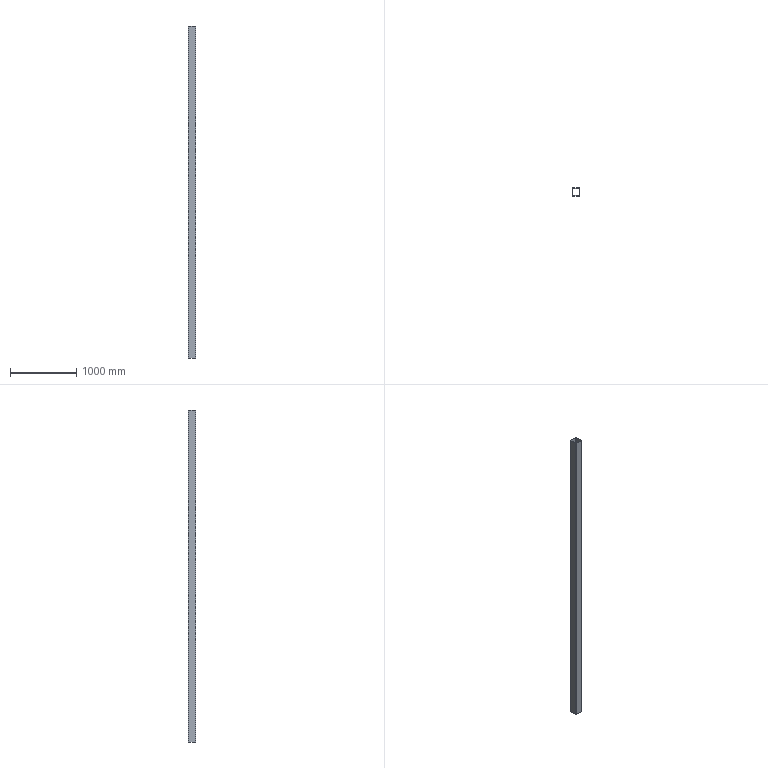Part | SolidWorks | features ICE 1, LibraryFeature 1 | 1 solid | 18 faces | box 120 x 120 x 5030 mm | volume 9128426 mm3 | plane 10 | cylinder 8 | commonest cylinder face diameters 8 x4 16 x4
STEP:
#1=CARTESIAN_POINT('',(52.,60.,-2515.));
#2=VERTEX_POINT('',#1);
#3=CARTESIAN_POINT('',(-52.,60.,-2515.));
#4=VERTEX_POINT('',#3);
#5=CARTESIAN_POINT('',(0.,60.,-2515.));
#6=DIRECTION('',(-1.,0.,0.));
#7=VECTOR('',#6,1000.);
#8=LINE('',#5,#7);
#9=EDGE_CURVE('',#2,#4,#8,.T.);
#10=ORIENTED_EDGE('',*,*,#9,.T.);
#11=CARTESIAN_POINT('',(-52.,60.,2515.));
#12=VERTEX_POINT('',#11);
#13=CARTESIAN_POINT('',(-52.,60.,2515.));
#14=DIRECTION('',(0.,0.,-1.));
#15=VECTOR('',#14,1000.);
#16=LINE('',#13,#15);
#17=EDGE_CURVE('',#12,#4,#16,.T.);
#18=ORIENTED_EDGE('',*,*,#17,.F.);
#19=CARTESIAN_POINT('',(52.,60.,2515.));
#20=VERTEX_POINT('',#19);
#21=CARTESIAN_POINT('',(0.,60.,2515.));
#22=DIRECTION('',(-1.,0.,0.));
#23=VECTOR('',#22,1000.);
#24=LINE('',#21,#23);
#25=EDGE_CURVE('',#20,#12,#24,.T.);
#26=ORIENTED_EDGE('',*,*,#25,.F.);
#27=CARTESIAN_POINT('',(52.,60.,2515.));
#28=DIRECTION('',(0.,0.,-1.));
#29=VECTOR('',#28,1000.);
#30=LINE('',#27,#29);
#31=EDGE_CURVE('',#20,#2,#30,.T.);
#32=ORIENTED_EDGE('',*,*,#31,.T.);
#33=EDGE_LOOP('',(#10,#18,#26,#32));
#34=FACE_OUTER_BOUND('',#33,.T.);
#35=CARTESIAN_POINT('',(0.,60.,2515.));
#36=DIRECTION('',(0.,-1.,0.));
#37=DIRECTION('',(0.,0.,-1.));
#38=AXIS2_PLACEMENT_3D('',#35,#36,#37);
#39=PLANE('',#38);
#40=ADVANCED_FACE('',(#34),#39,.F.);
#41=CARTESIAN_POINT('',(-60.,52.,-2515.));
#42=VERTEX_POINT('',#41);
#43=CARTESIAN_POINT('',(-52.,52.,-2515.));
#44=DIRECTION('',(0.,0.,1.));
#45=DIRECTION('',(1.,0.,0.));
#46=AXIS2_PLACEMENT_3D('',#43,#44,#45);
#47=CIRCLE('',#46,8.);
#48=EDGE_CURVE('',#4,#42,#47,.T.);
#49=ORIENTED_EDGE('',*,*,#48,.T.);
#50=CARTESIAN_POINT('',(-60.,52.,2515.));
#51=VERTEX_POINT('',#50);
#52=CARTESIAN_POINT('',(-60.,52.,2515.));
#53=DIRECTION('',(0.,0.,-1.));
#54=VECTOR('',#53,1000.);
#55=LINE('',#52,#54);
#56=EDGE_CURVE('',#51,#42,#55,.T.);
#57=ORIENTED_EDGE('',*,*,#56,.F.);
#58=CARTESIAN_POINT('',(-52.,52.,2515.));
#59=DIRECTION('',(0.,0.,1.));
#60=DIRECTION('',(1.,0.,0.));
#61=AXIS2_PLACEMENT_3D('',#58,#59,#60);
#62=CIRCLE('',#61,8.);
#63=EDGE_CURVE('',#12,#51,#62,.T.);
#64=ORIENTED_EDGE('',*,*,#63,.F.);
#65=ORIENTED_EDGE('',*,*,#17,.T.);
#66=EDGE_LOOP('',(#49,#57,#64,#65));
#67=FACE_OUTER_BOUND('',#66,.T.);
#68=CARTESIAN_POINT('',(-52.,52.,2515.));
#69=DIRECTION('',(0.,0.,-1.));
#70=DIRECTION('',(-1.,0.,0.));
#71=AXIS2_PLACEMENT_3D('',#68,#69,#70);
#72=CYLINDRICAL_SURFACE('',#71,8.);
#73=ADVANCED_FACE('',(#67),#72,.T.);
#74=CARTESIAN_POINT('',(-60.,-52.,-2515.));
#75=VERTEX_POINT('',#74);
#76=CARTESIAN_POINT('',(-60.,0.,-2515.));
#77=DIRECTION('',(0.,1.,0.));
#78=VECTOR('',#77,1000.);
#79=LINE('',#76,#78);
#80=EDGE_CURVE('',#75,#42,#79,.T.);
#81=ORIENTED_EDGE('',*,*,#80,.F.);
#82=CARTESIAN_POINT('',(-60.,-52.,2515.));
#83=VERTEX_POINT('',#82);
#84=CARTESIAN_POINT('',(-60.,-52.,2515.));
#85=DIRECTION('',(0.,0.,-1.));
#86=VECTOR('',#85,1000.);
#87=LINE('',#84,#86);
#88=EDGE_CURVE('',#83,#75,#87,.T.);
#89=ORIENTED_EDGE('',*,*,#88,.F.);
#90=CARTESIAN_POINT('',(-60.,0.,2515.));
#91=DIRECTION('',(0.,1.,0.));
#92=VECTOR('',#91,1000.);
#93=LINE('',#90,#92);
#94=EDGE_CURVE('',#83,#51,#93,.T.);
#95=ORIENTED_EDGE('',*,*,#94,.T.);
#96=ORIENTED_EDGE('',*,*,#56,.T.);
#97=EDGE_LOOP('',(#81,#89,#95,#96));
#98=FACE_OUTER_BOUND('',#97,.T.);
#99=CARTESIAN_POINT('',(-60.,0.,2515.));
#100=DIRECTION('',(-1.,0.,0.));
#101=DIRECTION('',(0.,0.,1.));
#102=AXIS2_PLACEMENT_3D('',#99,#100,#101);
#103=PLANE('',#102);
#104=ADVANCED_FACE('',(#98),#103,.T.);
#105=CARTESIAN_POINT('',(-52.,-60.,-2515.));
#106=VERTEX_POINT('',#105);
#107=CARTESIAN_POINT('',(-52.,-52.,-2515.));
#108=DIRECTION('',(0.,0.,1.));
#109=DIRECTION('',(1.,0.,0.));
#110=AXIS2_PLACEMENT_3D('',#107,#108,#109);
#111=CIRCLE('',#110,8.);
#112=EDGE_CURVE('',#75,#106,#111,.T.);
#113=ORIENTED_EDGE('',*,*,#112,.T.);
#114=CARTESIAN_POINT('',(-52.,-60.,2515.));
#115=VERTEX_POINT('',#114);
#116=CARTESIAN_POINT('',(-52.,-60.,2515.));
#117=DIRECTION('',(0.,0.,-1.));
#118=VECTOR('',#117,1000.);
#119=LINE('',#116,#118);
#120=EDGE_CURVE('',#115,#106,#119,.T.);
#121=ORIENTED_EDGE('',*,*,#120,.F.);
#122=CARTESIAN_POINT('',(-52.,-52.,2515.));
#123=DIRECTION('',(0.,0.,1.));
#124=DIRECTION('',(1.,0.,0.));
#125=AXIS2_PLACEMENT_3D('',#122,#123,#124);
#126=CIRCLE('',#125,8.);
#127=EDGE_CURVE('',#83,#115,#126,.T.);
#128=ORIENTED_EDGE('',*,*,#127,.F.);
#129=ORIENTED_EDGE('',*,*,#88,.T.);
#130=EDGE_LOOP('',(#113,#121,#128,#129));
#131=FACE_OUTER_BOUND('',#130,.T.);
#132=CARTESIAN_POINT('',(-52.,-52.,2515.));
#133=DIRECTION('',(0.,0.,-1.));
#134=DIRECTION('',(-1.,0.,0.));
#135=AXIS2_PLACEMENT_3D('',#132,#133,#134);
#136=CYLINDRICAL_SURFACE('',#135,8.);
#137=ADVANCED_FACE('',(#131),#136,.T.);
#138=CARTESIAN_POINT('',(52.,-60.,-2515.));
#139=VERTEX_POINT('',#138);
#140=CARTESIAN_POINT('',(0.,-60.,-2515.));
#141=DIRECTION('',(1.,0.,0.));
#142=VECTOR('',#141,1000.);
#143=LINE('',#140,#142);
#144=EDGE_CURVE('',#106,#139,#143,.T.);
#145=ORIENTED_EDGE('',*,*,#144,.T.);
#146=CARTESIAN_POINT('',(52.,-60.,2515.));
#147=VERTEX_POINT('',#146);
#148=CARTESIAN_POINT('',(52.,-60.,2515.));
#149=DIRECTION('',(0.,0.,-1.));
#150=VECTOR('',#149,1000.);
#151=LINE('',#148,#150);
#152=EDGE_CURVE('',#147,#139,#151,.T.);
#153=ORIENTED_EDGE('',*,*,#152,.F.);
#154=CARTESIAN_POINT('',(0.,-60.,2515.));
#155=DIRECTION('',(1.,0.,0.));
#156=VECTOR('',#155,1000.);
#157=LINE('',#154,#156);
#158=EDGE_CURVE('',#115,#147,#157,.T.);
#159=ORIENTED_EDGE('',*,*,#158,.F.);
#160=ORIENTED_EDGE('',*,*,#120,.T.);
#161=EDGE_LOOP('',(#145,#153,#159,#160));
#162=FACE_OUTER_BOUND('',#161,.T.);
#163=CARTESIAN_POINT('',(0.,-60.,2515.));
#164=DIRECTION('',(0.,1.,0.));
#165=DIRECTION('',(0.,0.,1.));
#166=AXIS2_PLACEMENT_3D('',#163,#164,#165);
#167=PLANE('',#166);
#168=ADVANCED_FACE('',(#162),#167,.F.);
#169=CARTESIAN_POINT('',(60.,-52.,-2515.));
#170=VERTEX_POINT('',#169);
#171=CARTESIAN_POINT('',(52.,-52.,-2515.));
#172=DIRECTION('',(0.,0.,1.));
#173=DIRECTION('',(1.,0.,0.));
#174=AXIS2_PLACEMENT_3D('',#171,#172,#173);
#175=CIRCLE('',#174,8.);
#176=EDGE_CURVE('',#139,#170,#175,.T.);
#177=ORIENTED_EDGE('',*,*,#176,.T.);
#178=CARTESIAN_POINT('',(60.,-52.,2515.));
#179=VERTEX_POINT('',#178);
#180=CARTESIAN_POINT('',(60.,-52.,2515.));
#181=DIRECTION('',(0.,0.,-1.));
#182=VECTOR('',#181,1000.);
#183=LINE('',#180,#182);
#184=EDGE_CURVE('',#179,#170,#183,.T.);
#185=ORIENTED_EDGE('',*,*,#184,.F.);
#186=CARTESIAN_POINT('',(52.,-52.,2515.));
#187=DIRECTION('',(0.,0.,1.));
#188=DIRECTION('',(1.,0.,0.));
#189=AXIS2_PLACEMENT_3D('',#186,#187,#188);
#190=CIRCLE('',#189,8.);
#191=EDGE_CURVE('',#147,#179,#190,.T.);
#192=ORIENTED_EDGE('',*,*,#191,.F.);
#193=ORIENTED_EDGE('',*,*,#152,.T.);
#194=EDGE_LOOP('',(#177,#185,#192,#193));
#195=FACE_OUTER_BOUND('',#194,.T.);
#196=CARTESIAN_POINT('',(52.,-52.,2515.));
#197=DIRECTION('',(0.,0.,-1.));
#198=DIRECTION('',(-1.,0.,0.));
#199=AXIS2_PLACEMENT_3D('',#196,#197,#198);
#200=CYLINDRICAL_SURFACE('',#199,8.);
#201=ADVANCED_FACE('',(#195),#200,.T.);
#202=CARTESIAN_POINT('',(60.,52.,-2515.));
#203=VERTEX_POINT('',#202);
#204=CARTESIAN_POINT('',(60.,0.,-2515.));
#205=DIRECTION('',(0.,-1.,0.));
#206=VECTOR('',#205,1000.);
#207=LINE('',#204,#206);
#208=EDGE_CURVE('',#203,#170,#207,.T.);
#209=ORIENTED_EDGE('',*,*,#208,.F.);
#210=CARTESIAN_POINT('',(60.,52.,2515.));
#211=VERTEX_POINT('',#210);
#212=CARTESIAN_POINT('',(60.,52.,2515.));
#213=DIRECTION('',(0.,0.,-1.));
#214=VECTOR('',#213,1000.);
#215=LINE('',#212,#214);
#216=EDGE_CURVE('',#211,#203,#215,.T.);
#217=ORIENTED_EDGE('',*,*,#216,.F.);
#218=CARTESIAN_POINT('',(60.,0.,2515.));
#219=DIRECTION('',(0.,-1.,0.));
#220=VECTOR('',#219,1000.);
#221=LINE('',#218,#220);
#222=EDGE_CURVE('',#211,#179,#221,.T.);
#223=ORIENTED_EDGE('',*,*,#222,.T.);
#224=ORIENTED_EDGE('',*,*,#184,.T.);
#225=EDGE_LOOP('',(#209,#217,#223,#224));
#226=FACE_OUTER_BOUND('',#225,.T.);
#227=CARTESIAN_POINT('',(60.,0.,2515.));
#228=DIRECTION('',(1.,0.,0.));
#229=DIRECTION('',(0.,0.,-1.));
#230=AXIS2_PLACEMENT_3D('',#227,#228,#229);
#231=PLANE('',#230);
#232=ADVANCED_FACE('',(#226),#231,.T.);
#233=CARTESIAN_POINT('',(-56.,-52.,-2515.));
#234=VERTEX_POINT('',#233);
#235=CARTESIAN_POINT('',(-52.,-56.,-2515.));
#236=VERTEX_POINT('',#235);
#237=CARTESIAN_POINT('',(-52.,-52.,-2515.));
#238=DIRECTION('',(0.,0.,1.));
#239=DIRECTION('',(1.,0.,0.));
#240=AXIS2_PLACEMENT_3D('',#237,#238,#239);
#241=CIRCLE('',#240,4.);
#242=EDGE_CURVE('',#234,#236,#241,.T.);
#243=ORIENTED_EDGE('',*,*,#242,.F.);
#244=CARTESIAN_POINT('',(-56.,-52.,2515.));
#245=VERTEX_POINT('',#244);
#246=CARTESIAN_POINT('',(-56.,-52.,2515.));
#247=DIRECTION('',(0.,0.,-1.));
#248=VECTOR('',#247,1000.);
#249=LINE('',#246,#248);
#250=EDGE_CURVE('',#245,#234,#249,.T.);
#251=ORIENTED_EDGE('',*,*,#250,.F.);
#252=CARTESIAN_POINT('',(-52.,-56.,2515.));
#253=VERTEX_POINT('',#252);
#254=CARTESIAN_POINT('',(-52.,-52.,2515.));
#255=DIRECTION('',(0.,0.,1.));
#256=DIRECTION('',(1.,0.,0.));
#257=AXIS2_PLACEMENT_3D('',#254,#255,#256);
#258=CIRCLE('',#257,4.);
#259=EDGE_CURVE('',#245,#253,#258,.T.);
#260=ORIENTED_EDGE('',*,*,#259,.T.);
#261=CARTESIAN_POINT('',(-52.,-56.,2515.));
#262=DIRECTION('',(0.,0.,-1.));
#263=VECTOR('',#262,1000.);
#264=LINE('',#261,#263);
#265=EDGE_CURVE('',#253,#236,#264,.T.);
#266=ORIENTED_EDGE('',*,*,#265,.T.);
#267=EDGE_LOOP('',(#243,#251,#260,#266));
#268=FACE_OUTER_BOUND('',#267,.T.);
#269=CARTESIAN_POINT('',(-52.,-52.,2515.));
#270=DIRECTION('',(0.,0.,-1.));
#271=DIRECTION('',(-1.,0.,0.));
#272=AXIS2_PLACEMENT_3D('',#269,#270,#271);
#273=CYLINDRICAL_SURFACE('',#272,4.);
#274=ADVANCED_FACE('',(#268),#273,.F.);
#275=CARTESIAN_POINT('',(-56.,52.,-2515.));
#276=VERTEX_POINT('',#275);
#277=CARTESIAN_POINT('',(-56.,0.,-2515.));
#278=DIRECTION('',(0.,1.,0.));
#279=VECTOR('',#278,1000.);
#280=LINE('',#277,#279);
#281=EDGE_CURVE('',#234,#276,#280,.T.);
#282=ORIENTED_EDGE('',*,*,#281,.T.);
#283=CARTESIAN_POINT('',(-56.,52.,2515.));
#284=VERTEX_POINT('',#283);
#285=CARTESIAN_POINT('',(-56.,52.,2515.));
#286=DIRECTION('',(0.,0.,-1.));
#287=VECTOR('',#286,1000.);
#288=LINE('',#285,#287);
#289=EDGE_CURVE('',#284,#276,#288,.T.);
#290=ORIENTED_EDGE('',*,*,#289,.F.);
#291=CARTESIAN_POINT('',(-56.,0.,2515.));
#292=DIRECTION('',(0.,1.,0.));
#293=VECTOR('',#292,1000.);
#294=LINE('',#291,#293);
#295=EDGE_CURVE('',#245,#284,#294,.T.);
#296=ORIENTED_EDGE('',*,*,#295,.F.);
#297=ORIENTED_EDGE('',*,*,#250,.T.);
#298=EDGE_LOOP('',(#282,#290,#296,#297));
#299=FACE_OUTER_BOUND('',#298,.T.);
#300=CARTESIAN_POINT('',(-56.,0.,2515.));
#301=DIRECTION('',(-1.,0.,0.));
#302=DIRECTION('',(0.,0.,1.));
#303=AXIS2_PLACEMENT_3D('',#300,#301,#302);
#304=PLANE('',#303);
#305=ADVANCED_FACE('',(#299),#304,.F.);
#306=CARTESIAN_POINT('',(-52.,56.,-2515.));
#307=VERTEX_POINT('',#306);
#308=CARTESIAN_POINT('',(-52.,52.,-2515.));
#309=DIRECTION('',(0.,0.,1.));
#310=DIRECTION('',(1.,0.,0.));
#311=AXIS2_PLACEMENT_3D('',#308,#309,#310);
#312=CIRCLE('',#311,4.);
#313=EDGE_CURVE('',#307,#276,#312,.T.);
#314=ORIENTED_EDGE('',*,*,#313,.F.);
#315=CARTESIAN_POINT('',(-52.,56.,2515.));
#316=VERTEX_POINT('',#315);
#317=CARTESIAN_POINT('',(-52.,56.,2515.));
#318=DIRECTION('',(0.,0.,-1.));
#319=VECTOR('',#318,1000.);
#320=LINE('',#317,#319);
#321=EDGE_CURVE('',#316,#307,#320,.T.);
#322=ORIENTED_EDGE('',*,*,#321,.F.);
#323=CARTESIAN_POINT('',(-52.,52.,2515.));
#324=DIRECTION('',(0.,0.,1.));
#325=DIRECTION('',(1.,0.,0.));
#326=AXIS2_PLACEMENT_3D('',#323,#324,#325);
#327=CIRCLE('',#326,4.);
#328=EDGE_CURVE('',#316,#284,#327,.T.);
#329=ORIENTED_EDGE('',*,*,#328,.T.);
#330=ORIENTED_EDGE('',*,*,#289,.T.);
#331=EDGE_LOOP('',(#314,#322,#329,#330));
#332=FACE_OUTER_BOUND('',#331,.T.);
#333=CARTESIAN_POINT('',(-52.,52.,2515.));
#334=DIRECTION('',(0.,0.,-1.));
#335=DIRECTION('',(-1.,0.,0.));
#336=AXIS2_PLACEMENT_3D('',#333,#334,#335);
#337=CYLINDRICAL_SURFACE('',#336,4.);
#338=ADVANCED_FACE('',(#332),#337,.F.);
#339=CARTESIAN_POINT('',(52.,56.,-2515.));
#340=VERTEX_POINT('',#339);
#341=CARTESIAN_POINT('',(0.,56.,-2515.));
#342=DIRECTION('',(-1.,0.,0.));
#343=VECTOR('',#342,1000.);
#344=LINE('',#341,#343);
#345=EDGE_CURVE('',#340,#307,#344,.T.);
#346=ORIENTED_EDGE('',*,*,#345,.F.);
#347=CARTESIAN_POINT('',(52.,56.,2515.));
#348=VERTEX_POINT('',#347);
#349=CARTESIAN_POINT('',(52.,56.,2515.));
#350=DIRECTION('',(0.,0.,-1.));
#351=VECTOR('',#350,1000.);
#352=LINE('',#349,#351);
#353=EDGE_CURVE('',#348,#340,#352,.T.);
#354=ORIENTED_EDGE('',*,*,#353,.F.);
#355=CARTESIAN_POINT('',(0.,56.,2515.));
#356=DIRECTION('',(-1.,0.,0.));
#357=VECTOR('',#356,1000.);
#358=LINE('',#355,#357);
#359=EDGE_CURVE('',#348,#316,#358,.T.);
#360=ORIENTED_EDGE('',*,*,#359,.T.);
#361=ORIENTED_EDGE('',*,*,#321,.T.);
#362=EDGE_LOOP('',(#346,#354,#360,#361));
#363=FACE_OUTER_BOUND('',#362,.T.);
#364=CARTESIAN_POINT('',(0.,56.,2515.));
#365=DIRECTION('',(0.,-1.,0.));
#366=DIRECTION('',(0.,0.,-1.));
#367=AXIS2_PLACEMENT_3D('',#364,#365,#366);
#368=PLANE('',#367);
#369=ADVANCED_FACE('',(#363),#368,.T.);
#370=CARTESIAN_POINT('',(56.,52.,-2515.));
#371=VERTEX_POINT('',#370);
#372=CARTESIAN_POINT('',(52.,52.,-2515.));
#373=DIRECTION('',(0.,0.,1.));
#374=DIRECTION('',(1.,0.,0.));
#375=AXIS2_PLACEMENT_3D('',#372,#373,#374);
#376=CIRCLE('',#375,4.);
#377=EDGE_CURVE('',#371,#340,#376,.T.);
#378=ORIENTED_EDGE('',*,*,#377,.F.);
#379=CARTESIAN_POINT('',(56.,52.,2515.));
#380=VERTEX_POINT('',#379);
#381=CARTESIAN_POINT('',(56.,52.,2515.));
#382=DIRECTION('',(0.,0.,-1.));
#383=VECTOR('',#382,1000.);
#384=LINE('',#381,#383);
#385=EDGE_CURVE('',#380,#371,#384,.T.);
#386=ORIENTED_EDGE('',*,*,#385,.F.);
#387=CARTESIAN_POINT('',(52.,52.,2515.));
#388=DIRECTION('',(0.,0.,1.));
#389=DIRECTION('',(1.,0.,0.));
#390=AXIS2_PLACEMENT_3D('',#387,#388,#389);
#391=CIRCLE('',#390,4.);
#392=EDGE_CURVE('',#380,#348,#391,.T.);
#393=ORIENTED_EDGE('',*,*,#392,.T.);
#394=ORIENTED_EDGE('',*,*,#353,.T.);
#395=EDGE_LOOP('',(#378,#386,#393,#394));
#396=FACE_OUTER_BOUND('',#395,.T.);
#397=CARTESIAN_POINT('',(52.,52.,2515.));
#398=DIRECTION('',(0.,0.,-1.));
#399=DIRECTION('',(-1.,0.,0.));
#400=AXIS2_PLACEMENT_3D('',#397,#398,#399);
#401=CYLINDRICAL_SURFACE('',#400,4.);
#402=ADVANCED_FACE('',(#396),#401,.F.);
#403=CARTESIAN_POINT('',(56.,-52.,-2515.));
#404=VERTEX_POINT('',#403);
#405=CARTESIAN_POINT('',(56.,0.,-2515.));
#406=DIRECTION('',(0.,-1.,0.));
#407=VECTOR('',#406,1000.);
#408=LINE('',#405,#407);
#409=EDGE_CURVE('',#371,#404,#408,.T.);
#410=ORIENTED_EDGE('',*,*,#409,.T.);
#411=CARTESIAN_POINT('',(56.,-52.,2515.));
#412=VERTEX_POINT('',#411);
#413=CARTESIAN_POINT('',(56.,-52.,2515.));
#414=DIRECTION('',(0.,0.,-1.));
#415=VECTOR('',#414,1000.);
#416=LINE('',#413,#415);
#417=EDGE_CURVE('',#412,#404,#416,.T.);
#418=ORIENTED_EDGE('',*,*,#417,.F.);
#419=CARTESIAN_POINT('',(56.,0.,2515.));
#420=DIRECTION('',(0.,-1.,0.));
#421=VECTOR('',#420,1000.);
#422=LINE('',#419,#421);
#423=EDGE_CURVE('',#380,#412,#422,.T.);
#424=ORIENTED_EDGE('',*,*,#423,.F.);
#425=ORIENTED_EDGE('',*,*,#385,.T.);
#426=EDGE_LOOP('',(#410,#418,#424,#425));
#427=FACE_OUTER_BOUND('',#426,.T.);
#428=CARTESIAN_POINT('',(56.,0.,2515.));
#429=DIRECTION('',(1.,0.,0.));
#430=DIRECTION('',(0.,0.,-1.));
#431=AXIS2_PLACEMENT_3D('',#428,#429,#430);
#432=PLANE('',#431);
#433=ADVANCED_FACE('',(#427),#432,.F.);
#434=CARTESIAN_POINT('',(52.,-56.,-2515.));
#435=VERTEX_POINT('',#434);
#436=CARTESIAN_POINT('',(52.,-52.,-2515.));
#437=DIRECTION('',(0.,0.,1.));
#438=DIRECTION('',(1.,0.,0.));
#439=AXIS2_PLACEMENT_3D('',#436,#437,#438);
#440=CIRCLE('',#439,4.);
#441=EDGE_CURVE('',#435,#404,#440,.T.);
#442=ORIENTED_EDGE('',*,*,#441,.F.);
#443=CARTESIAN_POINT('',(52.,-56.,2515.));
#444=VERTEX_POINT('',#443);
#445=CARTESIAN_POINT('',(52.,-56.,2515.));
#446=DIRECTION('',(0.,0.,-1.));
#447=VECTOR('',#446,1000.);
#448=LINE('',#445,#447);
#449=EDGE_CURVE('',#444,#435,#448,.T.);
#450=ORIENTED_EDGE('',*,*,#449,.F.);
#451=CARTESIAN_POINT('',(52.,-52.,2515.));
#452=DIRECTION('',(0.,0.,1.));
#453=DIRECTION('',(1.,0.,0.));
#454=AXIS2_PLACEMENT_3D('',#451,#452,#453);
#455=CIRCLE('',#454,4.);
#456=EDGE_CURVE('',#444,#412,#455,.T.);
#457=ORIENTED_EDGE('',*,*,#456,.T.);
#458=ORIENTED_EDGE('',*,*,#417,.T.);
#459=EDGE_LOOP('',(#442,#450,#457,#458));
#460=FACE_OUTER_BOUND('',#459,.T.);
#461=CARTESIAN_POINT('',(52.,-52.,2515.));
#462=DIRECTION('',(0.,0.,-1.));
#463=DIRECTION('',(-1.,0.,0.));
#464=AXIS2_PLACEMENT_3D('',#461,#462,#463);
#465=CYLINDRICAL_SURFACE('',#464,4.);
#466=ADVANCED_FACE('',(#460),#465,.F.);
#467=CARTESIAN_POINT('',(0.,-56.,-2515.));
#468=DIRECTION('',(1.,0.,0.));
#469=VECTOR('',#468,1000.);
#470=LINE('',#467,#469);
#471=EDGE_CURVE('',#236,#435,#470,.T.);
#472=ORIENTED_EDGE('',*,*,#471,.F.);
#473=ORIENTED_EDGE('',*,*,#265,.F.);
#474=CARTESIAN_POINT('',(0.,-56.,2515.));
#475=DIRECTION('',(1.,0.,0.));
#476=VECTOR('',#475,1000.);
#477=LINE('',#474,#476);
#478=EDGE_CURVE('',#253,#444,#477,.T.);
#479=ORIENTED_EDGE('',*,*,#478,.T.);
#480=ORIENTED_EDGE('',*,*,#449,.T.);
#481=EDGE_LOOP('',(#472,#473,#479,#480));
#482=FACE_OUTER_BOUND('',#481,.T.);
#483=CARTESIAN_POINT('',(0.,-56.,2515.));
#484=DIRECTION('',(0.,1.,0.));
#485=DIRECTION('',(0.,0.,1.));
#486=AXIS2_PLACEMENT_3D('',#483,#484,#485);
#487=PLANE('',#486);
#488=ADVANCED_FACE('',(#482),#487,.T.);
#489=CARTESIAN_POINT('',(52.,52.,-2515.));
#490=DIRECTION('',(0.,0.,1.));
#491=DIRECTION('',(1.,0.,0.));
#492=AXIS2_PLACEMENT_3D('',#489,#490,#491);
#493=CIRCLE('',#492,8.);
#494=EDGE_CURVE('',#203,#2,#493,.T.);
#495=ORIENTED_EDGE('',*,*,#494,.T.);
#496=ORIENTED_EDGE('',*,*,#31,.F.);
#497=CARTESIAN_POINT('',(52.,52.,2515.));
#498=DIRECTION('',(0.,0.,1.));
#499=DIRECTION('',(1.,0.,0.));
#500=AXIS2_PLACEMENT_3D('',#497,#498,#499);
#501=CIRCLE('',#500,8.);
#502=EDGE_CURVE('',#211,#20,#501,.T.);
#503=ORIENTED_EDGE('',*,*,#502,.F.);
#504=ORIENTED_EDGE('',*,*,#216,.T.);
#505=EDGE_LOOP('',(#495,#496,#503,#504));
#506=FACE_OUTER_BOUND('',#505,.T.);
#507=CARTESIAN_POINT('',(52.,52.,2515.));
#508=DIRECTION('',(0.,0.,-1.));
#509=DIRECTION('',(-1.,0.,0.));
#510=AXIS2_PLACEMENT_3D('',#507,#508,#509);
#511=CYLINDRICAL_SURFACE('',#510,8.);
#512=ADVANCED_FACE('',(#506),#511,.T.);
#513=ORIENTED_EDGE('',*,*,#259,.F.);
#514=ORIENTED_EDGE('',*,*,#295,.T.);
#515=ORIENTED_EDGE('',*,*,#328,.F.);
#516=ORIENTED_EDGE('',*,*,#359,.F.);
#517=ORIENTED_EDGE('',*,*,#392,.F.);
#518=ORIENTED_EDGE('',*,*,#423,.T.);
#519=ORIENTED_EDGE('',*,*,#456,.F.);
#520=ORIENTED_EDGE('',*,*,#478,.F.);
#521=EDGE_LOOP('',(#513,#514,#515,#516,#517,#518,#519,#520));
#522=FACE_BOUND('',#521,.T.);
#523=ORIENTED_EDGE('',*,*,#25,.T.);
#524=ORIENTED_EDGE('',*,*,#63,.T.);
#525=ORIENTED_EDGE('',*,*,#94,.F.);
#526=ORIENTED_EDGE('',*,*,#127,.T.);
#527=ORIENTED_EDGE('',*,*,#158,.T.);
#528=ORIENTED_EDGE('',*,*,#191,.T.);
#529=ORIENTED_EDGE('',*,*,#222,.F.);
#530=ORIENTED_EDGE('',*,*,#502,.T.);
#531=EDGE_LOOP('',(#523,#524,#525,#526,#527,#528,#529,#530));
#532=FACE_OUTER_BOUND('',#531,.T.);
#533=CARTESIAN_POINT('',(0.,0.,2515.));
#534=DIRECTION('',(0.,0.,1.));
#535=DIRECTION('',(1.,0.,0.));
#536=AXIS2_PLACEMENT_3D('',#533,#534,#535);
#537=PLANE('',#536);
#538=ADVANCED_FACE('',(#522,#532),#537,.T.);
#539=ORIENTED_EDGE('',*,*,#242,.T.);
#540=ORIENTED_EDGE('',*,*,#471,.T.);
#541=ORIENTED_EDGE('',*,*,#441,.T.);
#542=ORIENTED_EDGE('',*,*,#409,.F.);
#543=ORIENTED_EDGE('',*,*,#377,.T.);
#544=ORIENTED_EDGE('',*,*,#345,.T.);
#545=ORIENTED_EDGE('',*,*,#313,.T.);
#546=ORIENTED_EDGE('',*,*,#281,.F.);
#547=EDGE_LOOP('',(#539,#540,#541,#542,#543,#544,#545,#546));
#548=FACE_BOUND('',#547,.T.);
#549=ORIENTED_EDGE('',*,*,#9,.F.);
#550=ORIENTED_EDGE('',*,*,#494,.F.);
#551=ORIENTED_EDGE('',*,*,#208,.T.);
#552=ORIENTED_EDGE('',*,*,#176,.F.);
#553=ORIENTED_EDGE('',*,*,#144,.F.);
#554=ORIENTED_EDGE('',*,*,#112,.F.);
#555=ORIENTED_EDGE('',*,*,#80,.T.);
#556=ORIENTED_EDGE('',*,*,#48,.F.);
#557=EDGE_LOOP('',(#549,#550,#551,#552,#553,#554,#555,#556));
#558=FACE_OUTER_BOUND('',#557,.T.);
#559=CARTESIAN_POINT('',(0.,0.,-2515.));
#560=DIRECTION('',(0.,0.,1.));
#561=DIRECTION('',(1.,0.,0.));
#562=AXIS2_PLACEMENT_3D('',#559,#560,#561);
#563=PLANE('',#562);
#564=ADVANCED_FACE('',(#548,#558),#563,.F.);
#565=CLOSED_SHELL('',(#40,#73,#104,#137,#168,#201,#232,#274,#305,#338,#369,#402,#433,#466,#488,#512,#538,#564));
#566=MANIFOLD_SOLID_BREP('',#565);
#567=CARTESIAN_POINT('',(0.,0.,0.));
#568=DIRECTION('',(0.,0.,1.));
#569=DIRECTION('',(1.,0.,0.));
#570=AXIS2_PLACEMENT_3D('',#567,#568,#569);
#571=(LENGTH_UNIT()NAMED_UNIT(*)SI_UNIT(.MILLI.,.METRE.));
#572=UNCERTAINTY_MEASURE_WITH_UNIT(LENGTH_MEASURE(0.00001),#571,'','');
#573=(NAMED_UNIT(*)PLANE_ANGLE_UNIT()SI_UNIT($,.RADIAN.));
#574=(NAMED_UNIT(*)SI_UNIT($,.STERADIAN.)SOLID_ANGLE_UNIT());
#575=(GEOMETRIC_REPRESENTATION_CONTEXT(3)GLOBAL_UNCERTAINTY_ASSIGNED_CONTEXT((#572))GLOBAL_UNIT_ASSIGNED_CONTEXT((#571,#573,#574))REPRESENTATION_CONTEXT('',''));
#576=ADVANCED_BREP_SHAPE_REPRESENTATION('',(#566,#570),#575);